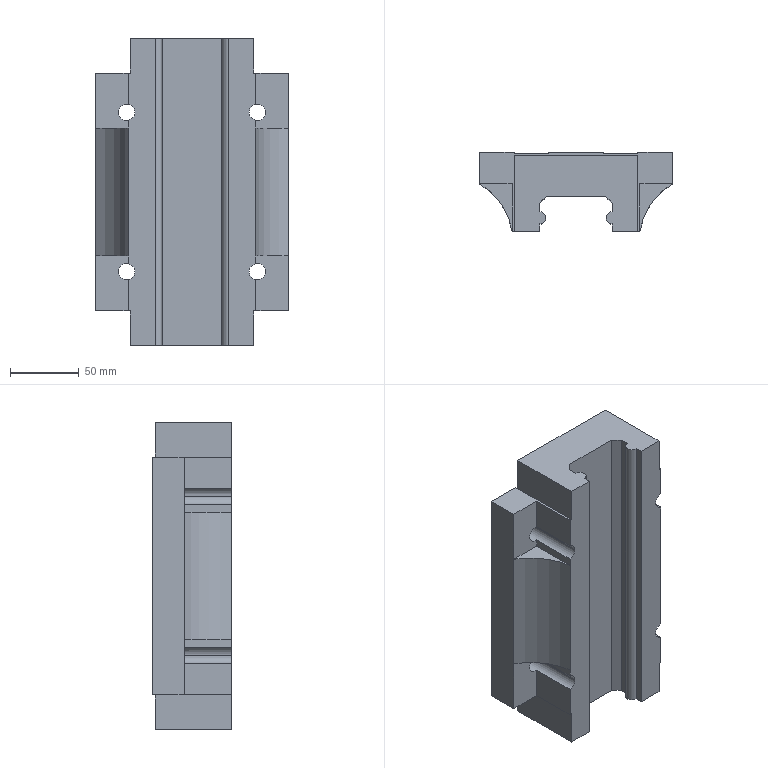Part | Creo | features CURVE 5, CUT 3, DATUM PLANE 3, PROTRUSION 3, COORDINATE SYSTEM 1, MIRROR 1 | 1 solid | 62 faces | box 140 x 57.3 x 223 mm | volume 1103476 mm3 | plane 50 | cylinder 12 | commonest cylinder face diameters 12 x8 8.877 x2 99.119 x2